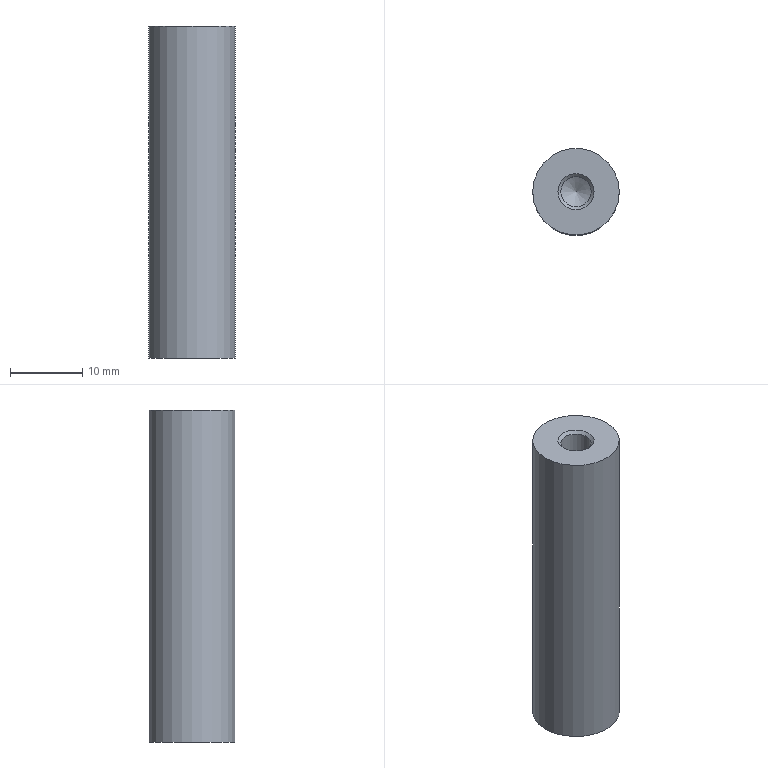Part | NX | 1 solid | 9 faces | box 12 x 12 x 46 mm | volume 4911 mm3 | cone 4 | cylinder 3 | plane 2 | commonest cylinder face diameters 4.2 x2 12 x1
STEP:
#1=CARTESIAN_POINT('',(6.,0.,0.));
#2=VERTEX_POINT('',#1);
#3=CARTESIAN_POINT('',(0.,0.,0.));
#4=DIRECTION('',(0.,0.,1.));
#5=DIRECTION('',(1.,0.,0.));
#6=AXIS2_PLACEMENT_3D('',#3,#4,#5);
#7=CIRCLE('',#6,6.);
#8=EDGE_CURVE('',#2,#2,#7,.T.);
#9=ORIENTED_EDGE('',*,*,#8,.T.);
#10=EDGE_LOOP('',(#9));
#11=FACE_BOUND('',#10,.T.);
#12=CARTESIAN_POINT('',(6.,0.,46.));
#13=VERTEX_POINT('',#12);
#14=CARTESIAN_POINT('',(0.,0.,46.));
#15=DIRECTION('',(0.,0.,1.));
#16=DIRECTION('',(1.,0.,0.));
#17=AXIS2_PLACEMENT_3D('',#14,#15,#16);
#18=CIRCLE('',#17,6.);
#19=EDGE_CURVE('',#13,#13,#18,.T.);
#20=ORIENTED_EDGE('',*,*,#19,.F.);
#21=EDGE_LOOP('',(#20));
#22=FACE_BOUND('',#21,.T.);
#23=CARTESIAN_POINT('',(0.,0.,46.));
#24=DIRECTION('',(0.,0.,-1.));
#25=DIRECTION('',(1.,0.,0.));
#26=AXIS2_PLACEMENT_3D('',#23,#24,#25);
#27=CYLINDRICAL_SURFACE('',#26,6.);
#28=ADVANCED_FACE('',(#11,#22),#27,.T.);
#29=CARTESIAN_POINT('',(2.5,0.,46.));
#30=VERTEX_POINT('',#29);
#31=CARTESIAN_POINT('',(0.,0.,46.));
#32=DIRECTION('',(0.,0.,-1.));
#33=DIRECTION('',(1.,0.,0.));
#34=AXIS2_PLACEMENT_3D('',#31,#32,#33);
#35=CIRCLE('',#34,2.5);
#36=EDGE_CURVE('',#30,#30,#35,.T.);
#37=ORIENTED_EDGE('',*,*,#36,.T.);
#38=EDGE_LOOP('',(#37));
#39=FACE_BOUND('',#38,.T.);
#40=ORIENTED_EDGE('',*,*,#19,.T.);
#41=EDGE_LOOP('',(#40));
#42=FACE_BOUND('',#41,.T.);
#43=CARTESIAN_POINT('',(0.,0.,46.));
#44=DIRECTION('',(0.,0.,1.));
#45=DIRECTION('',(-1.,0.,0.));
#46=AXIS2_PLACEMENT_3D('',#43,#44,#45);
#47=PLANE('',#46);
#48=ADVANCED_FACE('',(#39,#42),#47,.T.);
#49=CARTESIAN_POINT('',(2.5,0.,0.));
#50=VERTEX_POINT('',#49);
#51=CARTESIAN_POINT('',(0.,0.,0.));
#52=DIRECTION('',(0.,0.,1.));
#53=DIRECTION('',(1.,0.,0.));
#54=AXIS2_PLACEMENT_3D('',#51,#52,#53);
#55=CIRCLE('',#54,2.5);
#56=EDGE_CURVE('',#50,#50,#55,.T.);
#57=ORIENTED_EDGE('',*,*,#56,.T.);
#58=EDGE_LOOP('',(#57));
#59=FACE_BOUND('',#58,.T.);
#60=ORIENTED_EDGE('',*,*,#8,.F.);
#61=EDGE_LOOP('',(#60));
#62=FACE_BOUND('',#61,.T.);
#63=CARTESIAN_POINT('',(0.,0.,0.));
#64=DIRECTION('',(0.,0.,1.));
#65=DIRECTION('',(-1.,0.,0.));
#66=AXIS2_PLACEMENT_3D('',#63,#64,#65);
#67=PLANE('',#66);
#68=ADVANCED_FACE('',(#59,#62),#67,.F.);
#69=CARTESIAN_POINT('',(2.1,0.,10.));
#70=VERTEX_POINT('',#69);
#71=CARTESIAN_POINT('',(0.,0.,10.));
#72=DIRECTION('',(0.,0.,-1.));
#73=DIRECTION('',(1.,0.,0.));
#74=AXIS2_PLACEMENT_3D('',#71,#72,#73);
#75=CIRCLE('',#74,2.1);
#76=EDGE_CURVE('',#70,#70,#75,.T.);
#77=ORIENTED_EDGE('',*,*,#76,.T.);
#78=EDGE_LOOP('',(#77));
#79=FACE_BOUND('',#78,.T.);
#80=CARTESIAN_POINT('',(0.,0.,11.262));
#81=VERTEX_POINT('',#80);
#82=VERTEX_LOOP('',#81);
#83=FACE_BOUND('',#82,.T.);
#84=CARTESIAN_POINT('',(0.,0.,10.));
#85=DIRECTION('',(0.,0.,-1.));
#86=DIRECTION('',(1.,0.,0.));
#87=AXIS2_PLACEMENT_3D('',#84,#85,#86);
#88=CONICAL_SURFACE('',#87,2.1,59.);
#89=ADVANCED_FACE('',(#79,#83),#88,.F.);
#90=CARTESIAN_POINT('',(2.1,0.,0.4));
#91=VERTEX_POINT('',#90);
#92=CARTESIAN_POINT('',(0.,0.,0.4));
#93=DIRECTION('',(0.,0.,-1.));
#94=DIRECTION('',(1.,0.,0.));
#95=AXIS2_PLACEMENT_3D('',#92,#93,#94);
#96=CIRCLE('',#95,2.1);
#97=EDGE_CURVE('',#91,#91,#96,.T.);
#98=ORIENTED_EDGE('',*,*,#97,.T.);
#99=EDGE_LOOP('',(#98));
#100=FACE_BOUND('',#99,.T.);
#101=ORIENTED_EDGE('',*,*,#76,.F.);
#102=EDGE_LOOP('',(#101));
#103=FACE_BOUND('',#102,.T.);
#104=CARTESIAN_POINT('',(0.,0.,0.));
#105=DIRECTION('',(0.,0.,1.));
#106=DIRECTION('',(-1.,0.,0.));
#107=AXIS2_PLACEMENT_3D('',#104,#105,#106);
#108=CYLINDRICAL_SURFACE('',#107,2.1);
#109=ADVANCED_FACE('',(#100,#103),#108,.F.);
#110=ORIENTED_EDGE('',*,*,#97,.F.);
#111=EDGE_LOOP('',(#110));
#112=FACE_BOUND('',#111,.T.);
#113=ORIENTED_EDGE('',*,*,#56,.F.);
#114=EDGE_LOOP('',(#113));
#115=FACE_BOUND('',#114,.T.);
#116=CARTESIAN_POINT('',(0.,0.,0.));
#117=DIRECTION('',(0.,0.,-1.));
#118=DIRECTION('',(1.,0.,0.));
#119=AXIS2_PLACEMENT_3D('',#116,#117,#118);
#120=CONICAL_SURFACE('',#119,2.5,45.);
#121=ADVANCED_FACE('',(#112,#115),#120,.F.);
#122=CARTESIAN_POINT('',(-2.1,0.,36.));
#123=VERTEX_POINT('',#122);
#124=CARTESIAN_POINT('',(0.,0.,36.));
#125=DIRECTION('',(0.,0.,1.));
#126=DIRECTION('',(-1.,0.,0.));
#127=AXIS2_PLACEMENT_3D('',#124,#125,#126);
#128=CIRCLE('',#127,2.1);
#129=EDGE_CURVE('',#123,#123,#128,.T.);
#130=ORIENTED_EDGE('',*,*,#129,.T.);
#131=EDGE_LOOP('',(#130));
#132=FACE_BOUND('',#131,.T.);
#133=CARTESIAN_POINT('',(0.,0.,34.738));
#134=VERTEX_POINT('',#133);
#135=VERTEX_LOOP('',#134);
#136=FACE_BOUND('',#135,.T.);
#137=CARTESIAN_POINT('',(0.,0.,36.));
#138=DIRECTION('',(0.,0.,1.));
#139=DIRECTION('',(-1.,0.,0.));
#140=AXIS2_PLACEMENT_3D('',#137,#138,#139);
#141=CONICAL_SURFACE('',#140,2.1,59.);
#142=ADVANCED_FACE('',(#132,#136),#141,.F.);
#143=CARTESIAN_POINT('',(2.1,0.,45.6));
#144=VERTEX_POINT('',#143);
#145=CARTESIAN_POINT('',(0.,0.,45.6));
#146=DIRECTION('',(0.,0.,1.));
#147=DIRECTION('',(1.,0.,0.));
#148=AXIS2_PLACEMENT_3D('',#145,#146,#147);
#149=CIRCLE('',#148,2.1);
#150=EDGE_CURVE('',#144,#144,#149,.T.);
#151=ORIENTED_EDGE('',*,*,#150,.T.);
#152=EDGE_LOOP('',(#151));
#153=FACE_BOUND('',#152,.T.);
#154=ORIENTED_EDGE('',*,*,#129,.F.);
#155=EDGE_LOOP('',(#154));
#156=FACE_BOUND('',#155,.T.);
#157=CARTESIAN_POINT('',(0.,0.,46.));
#158=DIRECTION('',(0.,0.,-1.));
#159=DIRECTION('',(1.,0.,0.));
#160=AXIS2_PLACEMENT_3D('',#157,#158,#159);
#161=CYLINDRICAL_SURFACE('',#160,2.1);
#162=ADVANCED_FACE('',(#153,#156),#161,.F.);
#163=ORIENTED_EDGE('',*,*,#150,.F.);
#164=EDGE_LOOP('',(#163));
#165=FACE_BOUND('',#164,.T.);
#166=ORIENTED_EDGE('',*,*,#36,.F.);
#167=EDGE_LOOP('',(#166));
#168=FACE_BOUND('',#167,.T.);
#169=CARTESIAN_POINT('',(0.,0.,46.));
#170=DIRECTION('',(0.,0.,1.));
#171=DIRECTION('',(-1.,0.,0.));
#172=AXIS2_PLACEMENT_3D('',#169,#170,#171);
#173=CONICAL_SURFACE('',#172,2.5,45.);
#174=ADVANCED_FACE('',(#165,#168),#173,.F.);
#175=CLOSED_SHELL('',(#28,#48,#68,#89,#109,#121,#142,#162,#174));
#176=MANIFOLD_SOLID_BREP('',#175);
#177=(LENGTH_UNIT()NAMED_UNIT(*)SI_UNIT(.MILLI.,.METRE.));
#178=UNCERTAINTY_MEASURE_WITH_UNIT(LENGTH_MEASURE(0.00002),#177,'','');
#179=(NAMED_UNIT(*)PLANE_ANGLE_UNIT()SI_UNIT($,.RADIAN.));
#180=PLANE_ANGLE_MEASURE_WITH_UNIT(PLANE_ANGLE_MEASURE(0.01745),#179);
#181=DIMENSIONAL_EXPONENTS(0.,0.,0.,0.,0.,0.,0.);
#182=(CONVERSION_BASED_UNIT('DEGREE',#180)NAMED_UNIT(#181)PLANE_ANGLE_UNIT());
#183=(NAMED_UNIT(*)SI_UNIT($,.STERADIAN.)SOLID_ANGLE_UNIT());
#184=(GEOMETRIC_REPRESENTATION_CONTEXT(3)GLOBAL_UNCERTAINTY_ASSIGNED_CONTEXT((#178))GLOBAL_UNIT_ASSIGNED_CONTEXT((#177,#182,#183))REPRESENTATION_CONTEXT('',''));
#185=ADVANCED_BREP_SHAPE_REPRESENTATION('',(#176),#184);